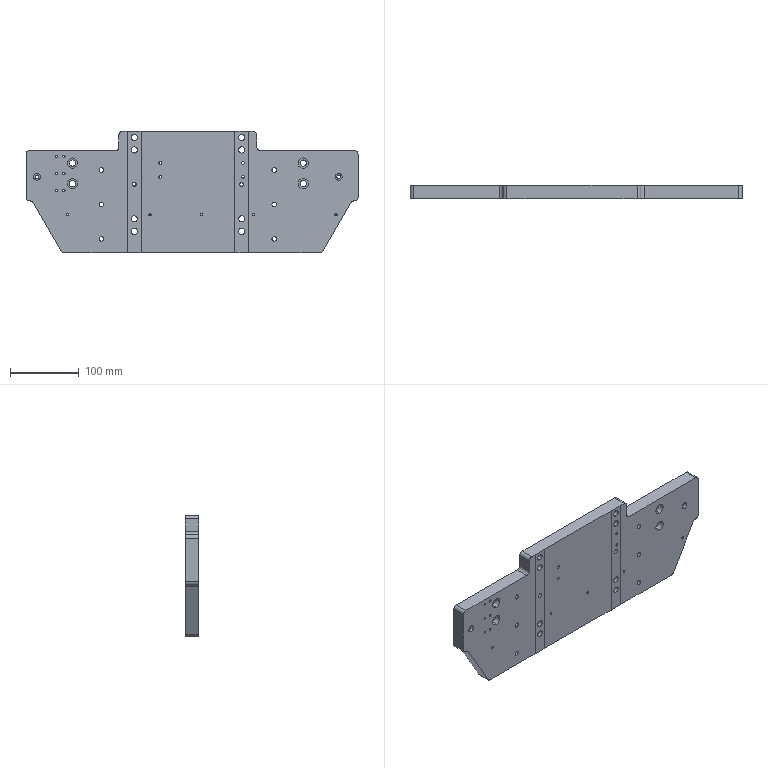Part | STEP file | 1 solid | 162 faces | box 482 x 20 x 176 mm | volume 1391575 mm3 | cylinder 122 | plane 40 | commonest cylinder face diameters 9 x24 15 x24 3.3 x22 10 x16 6.8 x12 4.2 x8